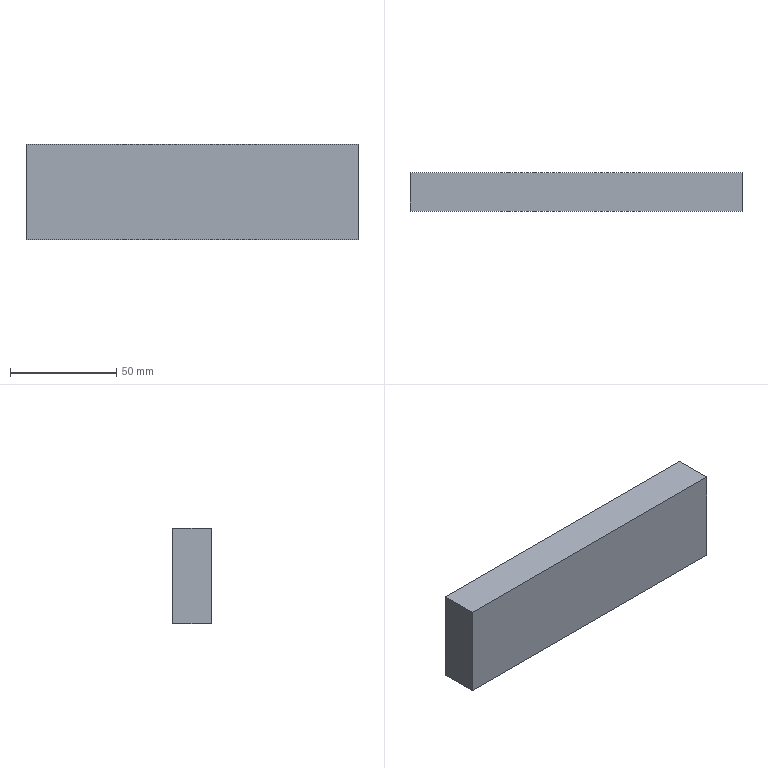Part | NX | 3 solids | 40 faces | box 156 x 18 x 45 mm | volume 213429 mm3 | plane 33 | cylinder 6 | spline 1 | commonest cylinder face diameters 6.5 x5 6 x1
STEP:
#1=CARTESIAN_POINT('',(180.,114.99,40.));
#2=VERTEX_POINT('',#1);
#3=CARTESIAN_POINT('',(30.,114.99,40.));
#4=VERTEX_POINT('',#3);
#5=CARTESIAN_POINT('',(105.,114.99,40.));
#6=DIRECTION('',(-1.,0.,0.));
#7=VECTOR('',#6,1000.);
#8=LINE('',#5,#7);
#9=EDGE_CURVE('',#2,#4,#8,.T.);
#10=ORIENTED_EDGE('',*,*,#9,.F.);
#11=CARTESIAN_POINT('',(180.,126.99,40.));
#12=VERTEX_POINT('',#11);
#13=CARTESIAN_POINT('',(180.,120.99,40.));
#14=DIRECTION('',(0.,-1.,0.));
#15=VECTOR('',#14,1000.);
#16=LINE('',#13,#15);
#17=EDGE_CURVE('',#12,#2,#16,.T.);
#18=ORIENTED_EDGE('',*,*,#17,.F.);
#19=CARTESIAN_POINT('',(30.,126.99,40.));
#20=VERTEX_POINT('',#19);
#21=CARTESIAN_POINT('',(105.,126.99,40.));
#22=DIRECTION('',(1.,0.,0.));
#23=VECTOR('',#22,1000.);
#24=LINE('',#21,#23);
#25=EDGE_CURVE('',#20,#12,#24,.T.);
#26=ORIENTED_EDGE('',*,*,#25,.F.);
#27=CARTESIAN_POINT('',(30.,120.99,40.));
#28=DIRECTION('',(0.,1.,0.));
#29=VECTOR('',#28,1000.);
#30=LINE('',#27,#29);
#31=EDGE_CURVE('',#4,#20,#30,.T.);
#32=ORIENTED_EDGE('',*,*,#31,.F.);
#33=EDGE_LOOP('',(#10,#18,#26,#32));
#34=FACE_BOUND('',#33,.T.);
#35=CARTESIAN_POINT('',(105.,120.99,40.));
#36=DIRECTION('',(0.,0.,1.));
#37=DIRECTION('',(1.,0.,0.));
#38=AXIS2_PLACEMENT_3D('',#35,#36,#37);
#39=PLANE('',#38);
#40=ADVANCED_FACE('',(#34),#39,.T.);
#41=CARTESIAN_POINT('',(180.,114.99,0.));
#42=VERTEX_POINT('',#41);
#43=CARTESIAN_POINT('',(180.,114.99,0.));
#44=DIRECTION('',(0.,0.,1.));
#45=VECTOR('',#44,1000.);
#46=LINE('',#43,#45);
#47=EDGE_CURVE('',#42,#2,#46,.T.);
#48=ORIENTED_EDGE('',*,*,#47,.T.);
#49=ORIENTED_EDGE('',*,*,#9,.T.);
#50=CARTESIAN_POINT('',(30.,114.99,0.));
#51=VERTEX_POINT('',#50);
#52=CARTESIAN_POINT('',(30.,114.99,0.));
#53=DIRECTION('',(0.,0.,1.));
#54=VECTOR('',#53,1000.);
#55=LINE('',#52,#54);
#56=EDGE_CURVE('',#51,#4,#55,.T.);
#57=ORIENTED_EDGE('',*,*,#56,.F.);
#58=CARTESIAN_POINT('',(105.,114.99,0.));
#59=DIRECTION('',(1.,0.,0.));
#60=VECTOR('',#59,1000.);
#61=LINE('',#58,#60);
#62=EDGE_CURVE('',#51,#42,#61,.T.);
#63=ORIENTED_EDGE('',*,*,#62,.T.);
#64=EDGE_LOOP('',(#48,#49,#57,#63));
#65=FACE_BOUND('',#64,.T.);
#66=CARTESIAN_POINT('',(105.,114.99,0.));
#67=DIRECTION('',(0.,-1.,0.));
#68=DIRECTION('',(0.,0.,-1.));
#69=AXIS2_PLACEMENT_3D('',#66,#67,#68);
#70=PLANE('',#69);
#71=ADVANCED_FACE('',(#65),#70,.T.);
#72=ORIENTED_EDGE('',*,*,#56,.T.);
#73=ORIENTED_EDGE('',*,*,#31,.T.);
#74=CARTESIAN_POINT('',(30.,126.99,0.));
#75=VERTEX_POINT('',#74);
#76=CARTESIAN_POINT('',(30.,126.99,0.));
#77=DIRECTION('',(0.,0.,1.));
#78=VECTOR('',#77,1000.);
#79=LINE('',#76,#78);
#80=EDGE_CURVE('',#75,#20,#79,.T.);
#81=ORIENTED_EDGE('',*,*,#80,.F.);
#82=CARTESIAN_POINT('',(30.,120.99,0.));
#83=DIRECTION('',(0.,-1.,0.));
#84=VECTOR('',#83,1000.);
#85=LINE('',#82,#84);
#86=EDGE_CURVE('',#75,#51,#85,.T.);
#87=ORIENTED_EDGE('',*,*,#86,.T.);
#88=EDGE_LOOP('',(#72,#73,#81,#87));
#89=FACE_BOUND('',#88,.T.);
#90=CARTESIAN_POINT('',(30.,120.99,0.));
#91=DIRECTION('',(-1.,0.,0.));
#92=DIRECTION('',(0.,0.,1.));
#93=AXIS2_PLACEMENT_3D('',#90,#91,#92);
#94=PLANE('',#93);
#95=ADVANCED_FACE('',(#89),#94,.T.);
#96=ORIENTED_EDGE('',*,*,#80,.T.);
#97=ORIENTED_EDGE('',*,*,#25,.T.);
#98=CARTESIAN_POINT('',(180.,126.99,0.));
#99=VERTEX_POINT('',#98);
#100=CARTESIAN_POINT('',(180.,126.99,0.));
#101=DIRECTION('',(0.,0.,1.));
#102=VECTOR('',#101,1000.);
#103=LINE('',#100,#102);
#104=EDGE_CURVE('',#99,#12,#103,.T.);
#105=ORIENTED_EDGE('',*,*,#104,.F.);
#106=CARTESIAN_POINT('',(105.,126.99,0.));
#107=DIRECTION('',(-1.,0.,0.));
#108=VECTOR('',#107,1000.);
#109=LINE('',#106,#108);
#110=EDGE_CURVE('',#99,#75,#109,.T.);
#111=ORIENTED_EDGE('',*,*,#110,.T.);
#112=EDGE_LOOP('',(#96,#97,#105,#111));
#113=FACE_BOUND('',#112,.T.);
#114=CARTESIAN_POINT('',(105.,126.99,0.));
#115=DIRECTION('',(0.,1.,0.));
#116=DIRECTION('',(0.,0.,1.));
#117=AXIS2_PLACEMENT_3D('',#114,#115,#116);
#118=PLANE('',#117);
#119=ADVANCED_FACE('',(#113),#118,.T.);
#120=CARTESIAN_POINT('',(180.,120.99,0.));
#121=DIRECTION('',(0.,1.,0.));
#122=VECTOR('',#121,1000.);
#123=LINE('',#120,#122);
#124=EDGE_CURVE('',#42,#99,#123,.T.);
#125=ORIENTED_EDGE('',*,*,#124,.F.);
#126=ORIENTED_EDGE('',*,*,#62,.F.);
#127=ORIENTED_EDGE('',*,*,#86,.F.);
#128=ORIENTED_EDGE('',*,*,#110,.F.);
#129=EDGE_LOOP('',(#125,#126,#127,#128));
#130=FACE_BOUND('',#129,.T.);
#131=CARTESIAN_POINT('',(105.,120.99,0.));
#132=DIRECTION('',(0.,0.,-1.));
#133=DIRECTION('',(-1.,0.,0.));
#134=AXIS2_PLACEMENT_3D('',#131,#132,#133);
#135=PLANE('',#134);
#136=ADVANCED_FACE('',(#130),#135,.T.);
#137=ORIENTED_EDGE('',*,*,#124,.T.);
#138=ORIENTED_EDGE('',*,*,#104,.T.);
#139=ORIENTED_EDGE('',*,*,#17,.T.);
#140=ORIENTED_EDGE('',*,*,#47,.F.);
#141=EDGE_LOOP('',(#137,#138,#139,#140));
#142=FACE_BOUND('',#141,.T.);
#143=CARTESIAN_POINT('',(180.,120.99,0.));
#144=DIRECTION('',(1.,0.,0.));
#145=DIRECTION('',(0.,0.,-1.));
#146=AXIS2_PLACEMENT_3D('',#143,#144,#145);
#147=PLANE('',#146);
#148=ADVANCED_FACE('',(#142),#147,.T.);
#149=CLOSED_SHELL('',(#40,#71,#95,#119,#136,#148));
#150=MANIFOLD_SOLID_BREP('',#149);
#151=CARTESIAN_POINT('',(175.75,115.12,7.));
#152=VERTEX_POINT('',#151);
#153=CARTESIAN_POINT('',(169.25,115.12,7.));
#154=VERTEX_POINT('',#153);
#155=CARTESIAN_POINT('',(172.5,115.12,7.));
#156=DIRECTION('',(0.,-1.,0.));
#157=DIRECTION('',(0.,0.,-1.));
#158=AXIS2_PLACEMENT_3D('',#155,#156,#157);
#159=CIRCLE('',#158,3.25);
#160=EDGE_CURVE('',#152,#154,#159,.F.);
#161=ORIENTED_EDGE('',*,*,#160,.T.);
#162=CARTESIAN_POINT('',(169.25,115.12,33.));
#163=VERTEX_POINT('',#162);
#164=CARTESIAN_POINT('',(169.25,115.12,13.));
#165=DIRECTION('',(0.,0.,1.));
#166=VECTOR('',#165,1000.);
#167=LINE('',#164,#166);
#168=EDGE_CURVE('',#154,#163,#167,.T.);
#169=ORIENTED_EDGE('',*,*,#168,.T.);
#170=CARTESIAN_POINT('',(175.75,115.12,33.));
#171=VERTEX_POINT('',#170);
#172=CARTESIAN_POINT('',(172.5,115.12,33.));
#173=DIRECTION('',(0.,-1.,0.));
#174=DIRECTION('',(0.,0.,-1.));
#175=AXIS2_PLACEMENT_3D('',#172,#173,#174);
#176=CIRCLE('',#175,3.25);
#177=EDGE_CURVE('',#163,#171,#176,.F.);
#178=ORIENTED_EDGE('',*,*,#177,.T.);
#179=CARTESIAN_POINT('',(175.75,115.12,13.));
#180=DIRECTION('',(0.,0.,-1.));
#181=VECTOR('',#180,1000.);
#182=LINE('',#179,#181);
#183=EDGE_CURVE('',#171,#152,#182,.T.);
#184=ORIENTED_EDGE('',*,*,#183,.T.);
#185=EDGE_LOOP('',(#161,#169,#178,#184));
#186=FACE_BOUND('',#185,.T.);
#187=CARTESIAN_POINT('',(165.,115.12,40.));
#188=VERTEX_POINT('',#187);
#189=CARTESIAN_POINT('',(179.,115.12,40.));
#190=VERTEX_POINT('',#189);
#191=CARTESIAN_POINT('',(158.,115.12,40.));
#192=DIRECTION('',(1.,0.,0.));
#193=VECTOR('',#192,1000.);
#194=LINE('',#191,#193);
#195=EDGE_CURVE('',#188,#190,#194,.T.);
#196=ORIENTED_EDGE('',*,*,#195,.F.);
#197=CARTESIAN_POINT('',(165.,115.12,0.));
#198=VERTEX_POINT('',#197);
#199=CARTESIAN_POINT('',(165.,115.12,13.));
#200=DIRECTION('',(0.,0.,-1.));
#201=VECTOR('',#200,1000.);
#202=LINE('',#199,#201);
#203=EDGE_CURVE('',#188,#198,#202,.T.);
#204=ORIENTED_EDGE('',*,*,#203,.T.);
#205=CARTESIAN_POINT('',(179.,115.12,0.));
#206=VERTEX_POINT('',#205);
#207=CARTESIAN_POINT('',(179.,115.12,0.));
#208=DIRECTION('',(-1.,0.,0.));
#209=VECTOR('',#208,1000.);
#210=LINE('',#207,#209);
#211=EDGE_CURVE('',#206,#198,#210,.T.);
#212=ORIENTED_EDGE('',*,*,#211,.F.);
#213=CARTESIAN_POINT('',(180.,115.12,1.));
#214=VERTEX_POINT('',#213);
#215=CARTESIAN_POINT('',(180.,115.12,1.));
#216=DIRECTION('',(-0.7071,0.,-0.7071));
#217=VECTOR('',#216,1000.);
#218=LINE('',#215,#217);
#219=EDGE_CURVE('',#214,#206,#218,.T.);
#220=ORIENTED_EDGE('',*,*,#219,.F.);
#221=CARTESIAN_POINT('',(180.,115.12,39.));
#222=VERTEX_POINT('',#221);
#223=CARTESIAN_POINT('',(180.,115.12,39.));
#224=DIRECTION('',(0.,0.,-1.));
#225=VECTOR('',#224,1000.);
#226=LINE('',#223,#225);
#227=EDGE_CURVE('',#222,#214,#226,.T.);
#228=ORIENTED_EDGE('',*,*,#227,.F.);
#229=CARTESIAN_POINT('',(179.,115.12,40.));
#230=DIRECTION('',(0.7071,0.,-0.7071));
#231=VECTOR('',#230,1000.);
#232=LINE('',#229,#231);
#233=EDGE_CURVE('',#190,#222,#232,.T.);
#234=ORIENTED_EDGE('',*,*,#233,.F.);
#235=EDGE_LOOP('',(#196,#204,#212,#220,#228,#234));
#236=FACE_BOUND('',#235,.T.);
#237=CARTESIAN_POINT('',(154.,115.12,13.));
#238=DIRECTION('',(0.,-1.,0.));
#239=DIRECTION('',(-1.,0.,0.));
#240=AXIS2_PLACEMENT_3D('',#237,#238,#239);
#241=PLANE('',#240);
#242=ADVANCED_FACE('',(#186,#236),#241,.T.);
#243=CARTESIAN_POINT('',(36.,124.24,0.));
#244=VERTEX_POINT('',#243);
#245=CARTESIAN_POINT('',(36.,117.74,0.));
#246=VERTEX_POINT('',#245);
#247=CARTESIAN_POINT('',(36.,120.99,0.));
#248=DIRECTION('',(0.,0.,1.));
#249=DIRECTION('',(1.,0.,0.));
#250=AXIS2_PLACEMENT_3D('',#247,#248,#249);
#251=CIRCLE('',#250,3.25);
#252=EDGE_CURVE('',#244,#246,#251,.T.);
#253=ORIENTED_EDGE('',*,*,#252,.T.);
#254=CARTESIAN_POINT('',(151.,117.74,0.));
#255=VERTEX_POINT('',#254);
#256=CARTESIAN_POINT('',(36.,117.74,0.));
#257=DIRECTION('',(1.,0.,0.));
#258=VECTOR('',#257,1000.);
#259=LINE('',#256,#258);
#260=EDGE_CURVE('',#246,#255,#259,.T.);
#261=ORIENTED_EDGE('',*,*,#260,.T.);
#262=CARTESIAN_POINT('',(154.,119.74,0.));
#263=VERTEX_POINT('',#262);
#264=CARTESIAN_POINT('',(151.,120.99,0.));
#265=DIRECTION('',(0.,0.,1.));
#266=DIRECTION('',(1.,0.,0.));
#267=AXIS2_PLACEMENT_3D('',#264,#265,#266);
#268=CIRCLE('',#267,3.25);
#269=EDGE_CURVE('',#255,#263,#268,.T.);
#270=ORIENTED_EDGE('',*,*,#269,.T.);
#271=CARTESIAN_POINT('',(154.,122.24,0.));
#272=VERTEX_POINT('',#271);
#273=CARTESIAN_POINT('',(154.,119.74,0.));
#274=CARTESIAN_POINT('',(154.165,120.14,0.));
#275=CARTESIAN_POINT('',(154.25,120.574,0.));
#276=CARTESIAN_POINT('',(154.25,121.406,0.));
#277=CARTESIAN_POINT('',(154.165,121.84,0.));
#278=CARTESIAN_POINT('',(154.,122.24,0.));
#279=B_SPLINE_CURVE_WITH_KNOTS('',3,(#273,#274,#275,#276,#277,#278),.UNSPECIFIED.,.F.,.F.,(4,2,4),(0.,0.5,1.),.UNSPECIFIED.);
#280=EDGE_CURVE('',#263,#272,#279,.T.);
#281=ORIENTED_EDGE('',*,*,#280,.T.);
#282=CARTESIAN_POINT('',(151.,124.24,0.));
#283=VERTEX_POINT('',#282);
#284=CARTESIAN_POINT('',(151.,120.99,0.));
#285=DIRECTION('',(0.,0.,1.));
#286=DIRECTION('',(1.,0.,0.));
#287=AXIS2_PLACEMENT_3D('',#284,#285,#286);
#288=CIRCLE('',#287,3.25);
#289=EDGE_CURVE('',#272,#283,#288,.T.);
#290=ORIENTED_EDGE('',*,*,#289,.T.);
#291=CARTESIAN_POINT('',(151.,124.24,0.));
#292=DIRECTION('',(-1.,0.,0.));
#293=VECTOR('',#292,1000.);
#294=LINE('',#291,#293);
#295=EDGE_CURVE('',#283,#244,#294,.T.);
#296=ORIENTED_EDGE('',*,*,#295,.T.);
#297=EDGE_LOOP('',(#253,#261,#270,#281,#290,#296));
#298=FACE_BOUND('',#297,.T.);
#299=ORIENTED_EDGE('',*,*,#211,.T.);
#300=CARTESIAN_POINT('',(165.,119.17,0.));
#301=VERTEX_POINT('',#300);
#302=CARTESIAN_POINT('',(165.,114.99,0.));
#303=DIRECTION('',(0.,1.,0.));
#304=VECTOR('',#303,1000.);
#305=LINE('',#302,#304);
#306=EDGE_CURVE('',#198,#301,#305,.T.);
#307=ORIENTED_EDGE('',*,*,#306,.T.);
#308=CARTESIAN_POINT('',(159.5,119.17,0.));
#309=VERTEX_POINT('',#308);
#310=CARTESIAN_POINT('',(179.,119.17,0.));
#311=DIRECTION('',(-1.,0.,0.));
#312=VECTOR('',#311,1000.);
#313=LINE('',#310,#312);
#314=EDGE_CURVE('',#301,#309,#313,.T.);
#315=ORIENTED_EDGE('',*,*,#314,.T.);
#316=CARTESIAN_POINT('',(159.5,114.99,0.));
#317=VERTEX_POINT('',#316);
#318=CARTESIAN_POINT('',(159.5,118.99,0.));
#319=DIRECTION('',(0.,-1.,0.));
#320=VECTOR('',#319,1000.);
#321=LINE('',#318,#320);
#322=EDGE_CURVE('',#309,#317,#321,.T.);
#323=ORIENTED_EDGE('',*,*,#322,.T.);
#324=CARTESIAN_POINT('',(31.,114.99,0.));
#325=VERTEX_POINT('',#324);
#326=CARTESIAN_POINT('',(179.,114.99,0.));
#327=DIRECTION('',(-1.,0.,0.));
#328=VECTOR('',#327,1000.);
#329=LINE('',#326,#328);
#330=EDGE_CURVE('',#317,#325,#329,.T.);
#331=ORIENTED_EDGE('',*,*,#330,.T.);
#332=CARTESIAN_POINT('',(31.,126.99,0.));
#333=VERTEX_POINT('',#332);
#334=CARTESIAN_POINT('',(31.,114.99,0.));
#335=DIRECTION('',(0.,1.,0.));
#336=VECTOR('',#335,1000.);
#337=LINE('',#334,#336);
#338=EDGE_CURVE('',#325,#333,#337,.T.);
#339=ORIENTED_EDGE('',*,*,#338,.T.);
#340=CARTESIAN_POINT('',(179.,126.99,0.));
#341=VERTEX_POINT('',#340);
#342=CARTESIAN_POINT('',(179.,126.99,0.));
#343=DIRECTION('',(-1.,0.,0.));
#344=VECTOR('',#343,1000.);
#345=LINE('',#342,#344);
#346=EDGE_CURVE('',#341,#333,#345,.T.);
#347=ORIENTED_EDGE('',*,*,#346,.F.);
#348=CARTESIAN_POINT('',(179.,114.99,0.));
#349=DIRECTION('',(0.,1.,0.));
#350=VECTOR('',#349,1000.);
#351=LINE('',#348,#350);
#352=EDGE_CURVE('',#206,#341,#351,.T.);
#353=ORIENTED_EDGE('',*,*,#352,.F.);
#354=EDGE_LOOP('',(#299,#307,#315,#323,#331,#339,#347,#353));
#355=FACE_BOUND('',#354,.T.);
#356=CARTESIAN_POINT('',(179.,114.99,0.));
#357=DIRECTION('',(0.,0.,-1.));
#358=DIRECTION('',(0.,1.,0.));
#359=AXIS2_PLACEMENT_3D('',#356,#357,#358);
#360=PLANE('',#359);
#361=ADVANCED_FACE('',(#298,#355),#360,.T.);
#362=CARTESIAN_POINT('',(154.,122.24,10.));
#363=VERTEX_POINT('',#362);
#364=CARTESIAN_POINT('',(154.,126.99,10.));
#365=VERTEX_POINT('',#364);
#366=CARTESIAN_POINT('',(154.,114.99,10.));
#367=DIRECTION('',(0.,1.,0.));
#368=VECTOR('',#367,1000.);
#369=LINE('',#366,#368);
#370=EDGE_CURVE('',#363,#365,#369,.T.);
#371=ORIENTED_EDGE('',*,*,#370,.F.);
#372=CARTESIAN_POINT('',(154.,119.74,10.));
#373=VERTEX_POINT('',#372);
#374=CARTESIAN_POINT('',(154.,122.24,10.));
#375=CARTESIAN_POINT('',(154.329,121.445,10.));
#376=CARTESIAN_POINT('',(154.329,120.536,10.));
#377=CARTESIAN_POINT('',(154.,119.74,10.));
#378=B_SPLINE_CURVE_WITH_KNOTS('',3,(#374,#375,#376,#377),.UNSPECIFIED.,.F.,.F.,(4,4),(0.,0.002569),.UNSPECIFIED.);
#379=EDGE_CURVE('',#363,#373,#378,.T.);
#380=ORIENTED_EDGE('',*,*,#379,.T.);
#381=CARTESIAN_POINT('',(154.,114.99,10.));
#382=VERTEX_POINT('',#381);
#383=CARTESIAN_POINT('',(154.,114.99,10.));
#384=DIRECTION('',(0.,1.,0.));
#385=VECTOR('',#384,1000.);
#386=LINE('',#383,#385);
#387=EDGE_CURVE('',#382,#373,#386,.T.);
#388=ORIENTED_EDGE('',*,*,#387,.F.);
#389=CARTESIAN_POINT('',(157.,114.99,13.));
#390=VERTEX_POINT('',#389);
#391=CARTESIAN_POINT('',(154.,114.99,13.));
#392=DIRECTION('',(0.,-1.,0.));
#393=DIRECTION('',(1.,0.,0.));
#394=AXIS2_PLACEMENT_3D('',#391,#392,#393);
#395=CIRCLE('',#394,3.);
#396=EDGE_CURVE('',#382,#390,#395,.T.);
#397=ORIENTED_EDGE('',*,*,#396,.T.);
#398=CARTESIAN_POINT('',(157.,126.99,13.));
#399=VERTEX_POINT('',#398);
#400=CARTESIAN_POINT('',(157.,114.99,13.));
#401=DIRECTION('',(0.,1.,0.));
#402=VECTOR('',#401,1000.);
#403=LINE('',#400,#402);
#404=EDGE_CURVE('',#390,#399,#403,.T.);
#405=ORIENTED_EDGE('',*,*,#404,.T.);
#406=CARTESIAN_POINT('',(154.,126.99,13.));
#407=DIRECTION('',(0.,-1.,0.));
#408=DIRECTION('',(1.,0.,0.));
#409=AXIS2_PLACEMENT_3D('',#406,#407,#408);
#410=CIRCLE('',#409,3.);
#411=EDGE_CURVE('',#365,#399,#410,.T.);
#412=ORIENTED_EDGE('',*,*,#411,.F.);
#413=EDGE_LOOP('',(#371,#380,#388,#397,#405,#412));
#414=FACE_BOUND('',#413,.T.);
#415=CARTESIAN_POINT('',(154.,114.99,13.));
#416=DIRECTION('',(0.,1.,0.));
#417=DIRECTION('',(1.,0.,0.));
#418=AXIS2_PLACEMENT_3D('',#415,#416,#417);
#419=CYLINDRICAL_SURFACE('',#418,3.);
#420=ADVANCED_FACE('',(#414),#419,.F.);
#421=ORIENTED_EDGE('',*,*,#387,.T.);
#422=CARTESIAN_POINT('',(151.,117.74,10.));
#423=VERTEX_POINT('',#422);
#424=CARTESIAN_POINT('',(151.,120.99,10.));
#425=DIRECTION('',(0.,0.,1.));
#426=DIRECTION('',(1.,0.,0.));
#427=AXIS2_PLACEMENT_3D('',#424,#425,#426);
#428=CIRCLE('',#427,3.25);
#429=EDGE_CURVE('',#373,#423,#428,.F.);
#430=ORIENTED_EDGE('',*,*,#429,.T.);
#431=CARTESIAN_POINT('',(36.,117.74,10.));
#432=VERTEX_POINT('',#431);
#433=CARTESIAN_POINT('',(31.,117.74,10.));
#434=DIRECTION('',(-1.,0.,0.));
#435=VECTOR('',#434,1000.);
#436=LINE('',#433,#435);
#437=EDGE_CURVE('',#423,#432,#436,.T.);
#438=ORIENTED_EDGE('',*,*,#437,.T.);
#439=CARTESIAN_POINT('',(36.,124.24,10.));
#440=VERTEX_POINT('',#439);
#441=CARTESIAN_POINT('',(36.,120.99,10.));
#442=DIRECTION('',(0.,0.,1.));
#443=DIRECTION('',(1.,0.,0.));
#444=AXIS2_PLACEMENT_3D('',#441,#442,#443);
#445=CIRCLE('',#444,3.25);
#446=EDGE_CURVE('',#432,#440,#445,.F.);
#447=ORIENTED_EDGE('',*,*,#446,.T.);
#448=CARTESIAN_POINT('',(151.,124.24,10.));
#449=VERTEX_POINT('',#448);
#450=CARTESIAN_POINT('',(31.,124.24,10.));
#451=DIRECTION('',(1.,0.,0.));
#452=VECTOR('',#451,1000.);
#453=LINE('',#450,#452);
#454=EDGE_CURVE('',#440,#449,#453,.T.);
#455=ORIENTED_EDGE('',*,*,#454,.T.);
#456=CARTESIAN_POINT('',(151.,120.99,10.));
#457=DIRECTION('',(0.,0.,1.));
#458=DIRECTION('',(1.,0.,0.));
#459=AXIS2_PLACEMENT_3D('',#456,#457,#458);
#460=CIRCLE('',#459,3.25);
#461=EDGE_CURVE('',#449,#363,#460,.F.);
#462=ORIENTED_EDGE('',*,*,#461,.T.);
#463=ORIENTED_EDGE('',*,*,#370,.T.);
#464=CARTESIAN_POINT('',(31.,126.99,10.));
#465=VERTEX_POINT('',#464);
#466=CARTESIAN_POINT('',(31.,126.99,10.));
#467=DIRECTION('',(1.,0.,0.));
#468=VECTOR('',#467,1000.);
#469=LINE('',#466,#468);
#470=EDGE_CURVE('',#465,#365,#469,.T.);
#471=ORIENTED_EDGE('',*,*,#470,.F.);
#472=CARTESIAN_POINT('',(31.,114.99,10.));
#473=VERTEX_POINT('',#472);
#474=CARTESIAN_POINT('',(31.,114.99,10.));
#475=DIRECTION('',(0.,1.,0.));
#476=VECTOR('',#475,1000.);
#477=LINE('',#474,#476);
#478=EDGE_CURVE('',#473,#465,#477,.T.);
#479=ORIENTED_EDGE('',*,*,#478,.F.);
#480=CARTESIAN_POINT('',(31.,114.99,10.));
#481=DIRECTION('',(1.,0.,0.));
#482=VECTOR('',#481,1000.);
#483=LINE('',#480,#482);
#484=EDGE_CURVE('',#473,#382,#483,.T.);
#485=ORIENTED_EDGE('',*,*,#484,.T.);
#486=EDGE_LOOP('',(#421,#430,#438,#447,#455,#462,#463,#471,#479,#485));
#487=FACE_BOUND('',#486,.T.);
#488=CARTESIAN_POINT('',(31.,114.99,10.));
#489=DIRECTION('',(0.,0.,1.));
#490=DIRECTION('',(1.,0.,0.));
#491=AXIS2_PLACEMENT_3D('',#488,#489,#490);
#492=PLANE('',#491);
#493=ADVANCED_FACE('',(#487),#492,.T.);
#494=CARTESIAN_POINT('',(157.,126.99,39.));
#495=VERTEX_POINT('',#494);
#496=CARTESIAN_POINT('',(157.,126.99,13.));
#497=DIRECTION('',(0.,0.,1.));
#498=VECTOR('',#497,1000.);
#499=LINE('',#496,#498);
#500=EDGE_CURVE('',#399,#495,#499,.T.);
#501=ORIENTED_EDGE('',*,*,#500,.F.);
#502=ORIENTED_EDGE('',*,*,#404,.F.);
#503=CARTESIAN_POINT('',(157.,114.99,39.));
#504=VERTEX_POINT('',#503);
#505=CARTESIAN_POINT('',(157.,114.99,13.));
#506=DIRECTION('',(0.,0.,1.));
#507=VECTOR('',#506,1000.);
#508=LINE('',#505,#507);
#509=EDGE_CURVE('',#390,#504,#508,.T.);
#510=ORIENTED_EDGE('',*,*,#509,.T.);
#511=CARTESIAN_POINT('',(157.,114.99,39.));
#512=DIRECTION('',(0.,1.,0.));
#513=VECTOR('',#512,1000.);
#514=LINE('',#511,#513);
#515=EDGE_CURVE('',#504,#495,#514,.T.);
#516=ORIENTED_EDGE('',*,*,#515,.T.);
#517=EDGE_LOOP('',(#501,#502,#510,#516));
#518=FACE_BOUND('',#517,.T.);
#519=CARTESIAN_POINT('',(157.,114.99,13.));
#520=DIRECTION('',(-1.,0.,0.));
#521=DIRECTION('',(0.,1.,0.));
#522=AXIS2_PLACEMENT_3D('',#519,#520,#521);
#523=PLANE('',#522);
#524=ADVANCED_FACE('',(#518),#523,.T.);
#525=CARTESIAN_POINT('',(158.,126.99,40.));
#526=VERTEX_POINT('',#525);
#527=CARTESIAN_POINT('',(157.,126.99,39.));
#528=DIRECTION('',(0.7071,0.,0.7071));
#529=VECTOR('',#528,1000.);
#530=LINE('',#527,#529);
#531=EDGE_CURVE('',#495,#526,#530,.T.);
#532=ORIENTED_EDGE('',*,*,#531,.F.);
#533=ORIENTED_EDGE('',*,*,#515,.F.);
#534=CARTESIAN_POINT('',(158.,114.99,40.));
#535=VERTEX_POINT('',#534);
#536=CARTESIAN_POINT('',(157.,114.99,39.));
#537=DIRECTION('',(0.7071,0.,0.7071));
#538=VECTOR('',#537,1000.);
#539=LINE('',#536,#538);
#540=EDGE_CURVE('',#504,#535,#539,.T.);
#541=ORIENTED_EDGE('',*,*,#540,.T.);
#542=CARTESIAN_POINT('',(158.,114.99,40.));
#543=DIRECTION('',(0.,1.,0.));
#544=VECTOR('',#543,1000.);
#545=LINE('',#542,#544);
#546=EDGE_CURVE('',#535,#526,#545,.T.);
#547=ORIENTED_EDGE('',*,*,#546,.T.);
#548=EDGE_LOOP('',(#532,#533,#541,#547));
#549=FACE_BOUND('',#548,.T.);
#550=CARTESIAN_POINT('',(157.,114.99,39.));
#551=DIRECTION('',(-0.7071,0.,0.7071));
#552=DIRECTION('',(0.7071,0.,0.7071));
#553=AXIS2_PLACEMENT_3D('',#550,#551,#552);
#554=PLANE('',#553);
#555=ADVANCED_FACE('',(#549),#554,.T.);
#556=CARTESIAN_POINT('',(159.5,119.17,40.));
#557=VERTEX_POINT('',#556);
#558=CARTESIAN_POINT('',(159.5,114.99,40.));
#559=VERTEX_POINT('',#558);
#560=CARTESIAN_POINT('',(159.5,118.99,40.));
#561=DIRECTION('',(0.,-1.,0.));
#562=VECTOR('',#561,1000.);
#563=LINE('',#560,#562);
#564=EDGE_CURVE('',#557,#559,#563,.T.);
#565=ORIENTED_EDGE('',*,*,#564,.F.);
#566=CARTESIAN_POINT('',(165.,119.17,40.));
#567=VERTEX_POINT('',#566);
#568=CARTESIAN_POINT('',(165.,119.17,40.));
#569=DIRECTION('',(-1.,0.,0.));
#570=VECTOR('',#569,1000.);
#571=LINE('',#568,#570);
#572=EDGE_CURVE('',#567,#557,#571,.T.);
#573=ORIENTED_EDGE('',*,*,#572,.F.);
#574=CARTESIAN_POINT('',(165.,114.99,40.));
#575=DIRECTION('',(0.,1.,0.));
#576=VECTOR('',#575,1000.);
#577=LINE('',#574,#576);
#578=EDGE_CURVE('',#188,#567,#577,.T.);
#579=ORIENTED_EDGE('',*,*,#578,.F.);
#580=ORIENTED_EDGE('',*,*,#195,.T.);
#581=CARTESIAN_POINT('',(179.,126.99,40.));
#582=VERTEX_POINT('',#581);
#583=CARTESIAN_POINT('',(179.,114.99,40.));
#584=DIRECTION('',(0.,1.,0.));
#585=VECTOR('',#584,1000.);
#586=LINE('',#583,#585);
#587=EDGE_CURVE('',#190,#582,#586,.T.);
#588=ORIENTED_EDGE('',*,*,#587,.T.);
#589=CARTESIAN_POINT('',(158.,126.99,40.));
#590=DIRECTION('',(1.,0.,0.));
#591=VECTOR('',#590,1000.);
#592=LINE('',#589,#591);
#593=EDGE_CURVE('',#526,#582,#592,.T.);
#594=ORIENTED_EDGE('',*,*,#593,.F.);
#595=ORIENTED_EDGE('',*,*,#546,.F.);
#596=CARTESIAN_POINT('',(158.,114.99,40.));
#597=DIRECTION('',(1.,0.,0.));
#598=VECTOR('',#597,1000.);
#599=LINE('',#596,#598);
#600=EDGE_CURVE('',#535,#559,#599,.T.);
#601=ORIENTED_EDGE('',*,*,#600,.T.);
#602=EDGE_LOOP('',(#565,#573,#579,#580,#588,#594,#595,#601));
#603=FACE_BOUND('',#602,.T.);
#604=CARTESIAN_POINT('',(158.,114.99,40.));
#605=DIRECTION('',(0.,0.,1.));
#606=DIRECTION('',(0.,-1.,0.));
#607=AXIS2_PLACEMENT_3D('',#604,#605,#606);
#608=PLANE('',#607);
#609=ADVANCED_FACE('',(#603),#608,.T.);
#610=CARTESIAN_POINT('',(180.,126.99,39.));
#611=VERTEX_POINT('',#610);
#612=CARTESIAN_POINT('',(179.,126.99,40.));
#613=DIRECTION('',(0.7071,0.,-0.7071));
#614=VECTOR('',#613,1000.);
#615=LINE('',#612,#614);
#616=EDGE_CURVE('',#582,#611,#615,.T.);
#617=ORIENTED_EDGE('',*,*,#616,.F.);
#618=ORIENTED_EDGE('',*,*,#587,.F.);
#619=ORIENTED_EDGE('',*,*,#233,.T.);
#620=CARTESIAN_POINT('',(180.,114.99,39.));
#621=DIRECTION('',(0.,1.,0.));
#622=VECTOR('',#621,1000.);
#623=LINE('',#620,#622);
#624=EDGE_CURVE('',#222,#611,#623,.T.);
#625=ORIENTED_EDGE('',*,*,#624,.T.);
#626=EDGE_LOOP('',(#617,#618,#619,#625));
#627=FACE_BOUND('',#626,.T.);
#628=CARTESIAN_POINT('',(179.,114.99,40.));
#629=DIRECTION('',(0.7071,0.,0.7071));
#630=DIRECTION('',(0.7071,0.,-0.7071));
#631=AXIS2_PLACEMENT_3D('',#628,#629,#630);
#632=PLANE('',#631);
#633=ADVANCED_FACE('',(#627),#632,.T.);
#634=CARTESIAN_POINT('',(180.,126.99,1.));
#635=VERTEX_POINT('',#634);
#636=CARTESIAN_POINT('',(180.,126.99,39.));
#637=DIRECTION('',(0.,0.,-1.));
#638=VECTOR('',#637,1000.);
#639=LINE('',#636,#638);
#640=EDGE_CURVE('',#611,#635,#639,.T.);
#641=ORIENTED_EDGE('',*,*,#640,.F.);
#642=ORIENTED_EDGE('',*,*,#624,.F.);
#643=ORIENTED_EDGE('',*,*,#227,.T.);
#644=CARTESIAN_POINT('',(180.,114.99,1.));
#645=DIRECTION('',(0.,1.,0.));
#646=VECTOR('',#645,1000.);
#647=LINE('',#644,#646);
#648=EDGE_CURVE('',#214,#635,#647,.T.);
#649=ORIENTED_EDGE('',*,*,#648,.T.);
#650=EDGE_LOOP('',(#641,#642,#643,#649));
#651=FACE_BOUND('',#650,.T.);
#652=CARTESIAN_POINT('',(180.,114.99,39.));
#653=DIRECTION('',(1.,0.,0.));
#654=DIRECTION('',(0.,-1.,0.));
#655=AXIS2_PLACEMENT_3D('',#652,#653,#654);
#656=PLANE('',#655);
#657=ADVANCED_FACE('',(#651),#656,.T.);
#658=CARTESIAN_POINT('',(180.,126.99,1.));
#659=DIRECTION('',(-0.7071,0.,-0.7071));
#660=VECTOR('',#659,1000.);
#661=LINE('',#658,#660);
#662=EDGE_CURVE('',#635,#341,#661,.T.);
#663=ORIENTED_EDGE('',*,*,#662,.F.);
#664=ORIENTED_EDGE('',*,*,#648,.F.);
#665=ORIENTED_EDGE('',*,*,#219,.T.);
#666=ORIENTED_EDGE('',*,*,#352,.T.);
#667=EDGE_LOOP('',(#663,#664,#665,#666));
#668=FACE_BOUND('',#667,.T.);
#669=CARTESIAN_POINT('',(180.,114.99,1.));
#670=DIRECTION('',(0.7071,0.,-0.7071));
#671=DIRECTION('',(-0.7071,0.,-0.7071));
#672=AXIS2_PLACEMENT_3D('',#669,#670,#671);
#673=PLANE('',#672);
#674=ADVANCED_FACE('',(#668),#673,.T.);
#675=CARTESIAN_POINT('',(30.,126.99,1.));
#676=VERTEX_POINT('',#675);
#677=CARTESIAN_POINT('',(31.,126.99,0.));
#678=DIRECTION('',(-0.7071,0.,0.7071));
#679=VECTOR('',#678,1000.);
#680=LINE('',#677,#679);
#681=EDGE_CURVE('',#333,#676,#680,.T.);
#682=ORIENTED_EDGE('',*,*,#681,.F.);
#683=ORIENTED_EDGE('',*,*,#338,.F.);
#684=CARTESIAN_POINT('',(30.,114.99,1.));
#685=VERTEX_POINT('',#684);
#686=CARTESIAN_POINT('',(31.,114.99,0.));
#687=DIRECTION('',(-0.7071,0.,0.7071));
#688=VECTOR('',#687,1000.);
#689=LINE('',#686,#688);
#690=EDGE_CURVE('',#325,#685,#689,.T.);
#691=ORIENTED_EDGE('',*,*,#690,.T.);
#692=CARTESIAN_POINT('',(30.,114.99,1.));
#693=DIRECTION('',(0.,1.,0.));
#694=VECTOR('',#693,1000.);
#695=LINE('',#692,#694);
#696=EDGE_CURVE('',#685,#676,#695,.T.);
#697=ORIENTED_EDGE('',*,*,#696,.T.);
#698=EDGE_LOOP('',(#682,#683,#691,#697));
#699=FACE_BOUND('',#698,.T.);
#700=CARTESIAN_POINT('',(31.,114.99,0.));
#701=DIRECTION('',(-0.7071,0.,-0.7071));
#702=DIRECTION('',(-0.7071,0.,0.7071));
#703=AXIS2_PLACEMENT_3D('',#700,#701,#702);
#704=PLANE('',#703);
#705=ADVANCED_FACE('',(#699),#704,.T.);
#706=CARTESIAN_POINT('',(30.,126.99,9.));
#707=VERTEX_POINT('',#706);
#708=CARTESIAN_POINT('',(30.,126.99,1.));
#709=DIRECTION('',(0.,0.,1.));
#710=VECTOR('',#709,1000.);
#711=LINE('',#708,#710);
#712=EDGE_CURVE('',#676,#707,#711,.T.);
#713=ORIENTED_EDGE('',*,*,#712,.F.);
#714=ORIENTED_EDGE('',*,*,#696,.F.);
#715=CARTESIAN_POINT('',(30.,114.99,9.));
#716=VERTEX_POINT('',#715);
#717=CARTESIAN_POINT('',(30.,114.99,1.));
#718=DIRECTION('',(0.,0.,1.));
#719=VECTOR('',#718,1000.);
#720=LINE('',#717,#719);
#721=EDGE_CURVE('',#685,#716,#720,.T.);
#722=ORIENTED_EDGE('',*,*,#721,.T.);
#723=CARTESIAN_POINT('',(30.,114.99,9.));
#724=DIRECTION('',(0.,1.,0.));
#725=VECTOR('',#724,1000.);
#726=LINE('',#723,#725);
#727=EDGE_CURVE('',#716,#707,#726,.T.);
#728=ORIENTED_EDGE('',*,*,#727,.T.);
#729=EDGE_LOOP('',(#713,#714,#722,#728));
#730=FACE_BOUND('',#729,.T.);
#731=CARTESIAN_POINT('',(30.,114.99,1.));
#732=DIRECTION('',(-1.,0.,0.));
#733=DIRECTION('',(0.,1.,0.));
#734=AXIS2_PLACEMENT_3D('',#731,#732,#733);
#735=PLANE('',#734);
#736=ADVANCED_FACE('',(#730),#735,.T.);
#737=CARTESIAN_POINT('',(30.,126.99,9.));
#738=DIRECTION('',(0.7071,0.,0.7071));
#739=VECTOR('',#738,1000.);
#740=LINE('',#737,#739);
#741=EDGE_CURVE('',#707,#465,#740,.T.);
#742=ORIENTED_EDGE('',*,*,#741,.F.);
#743=ORIENTED_EDGE('',*,*,#727,.F.);
#744=CARTESIAN_POINT('',(30.,114.99,9.));
#745=DIRECTION('',(0.7071,0.,0.7071));
#746=VECTOR('',#745,1000.);
#747=LINE('',#744,#746);
#748=EDGE_CURVE('',#716,#473,#747,.T.);
#749=ORIENTED_EDGE('',*,*,#748,.T.);
#750=ORIENTED_EDGE('',*,*,#478,.T.);
#751=EDGE_LOOP('',(#742,#743,#749,#750));
#752=FACE_BOUND('',#751,.T.);
#753=CARTESIAN_POINT('',(30.,114.99,9.));
#754=DIRECTION('',(-0.7071,0.,0.7071));
#755=DIRECTION('',(0.7071,0.,0.7071));
#756=AXIS2_PLACEMENT_3D('',#753,#754,#755);
#757=PLANE('',#756);
#758=ADVANCED_FACE('',(#752),#757,.T.);
#759=CARTESIAN_POINT('',(159.5,114.99,40.));
#760=DIRECTION('',(0.,0.,-1.));
#761=VECTOR('',#760,1000.);
#762=LINE('',#759,#761);
#763=EDGE_CURVE('',#559,#317,#762,.T.);
#764=ORIENTED_EDGE('',*,*,#763,.F.);
#765=ORIENTED_EDGE('',*,*,#600,.F.);
#766=ORIENTED_EDGE('',*,*,#540,.F.);
#767=ORIENTED_EDGE('',*,*,#509,.F.);
#768=ORIENTED_EDGE('',*,*,#396,.F.);
#769=ORIENTED_EDGE('',*,*,#484,.F.);
#770=ORIENTED_EDGE('',*,*,#748,.F.);
#771=ORIENTED_EDGE('',*,*,#721,.F.);
#772=ORIENTED_EDGE('',*,*,#690,.F.);
#773=ORIENTED_EDGE('',*,*,#330,.F.);
#774=EDGE_LOOP('',(#764,#765,#766,#767,#768,#769,#770,#771,#772,#773));
#775=FACE_BOUND('',#774,.T.);
#776=CARTESIAN_POINT('',(154.,114.99,13.));
#777=DIRECTION('',(0.,-1.,0.));
#778=DIRECTION('',(-1.,0.,0.));
#779=AXIS2_PLACEMENT_3D('',#776,#777,#778);
#780=PLANE('',#779);
#781=ADVANCED_FACE('',(#775),#780,.T.);
#782=CARTESIAN_POINT('',(169.25,126.99,33.));
#783=VERTEX_POINT('',#782);
#784=CARTESIAN_POINT('',(169.25,126.99,7.));
#785=VERTEX_POINT('',#784);
#786=CARTESIAN_POINT('',(169.25,126.99,33.));
#787=DIRECTION('',(0.,0.,-1.));
#788=VECTOR('',#787,1000.);
#789=LINE('',#786,#788);
#790=EDGE_CURVE('',#783,#785,#789,.T.);
#791=ORIENTED_EDGE('',*,*,#790,.T.);
#792=CARTESIAN_POINT('',(175.75,126.99,7.));
#793=VERTEX_POINT('',#792);
#794=CARTESIAN_POINT('',(172.5,126.99,7.));
#795=DIRECTION('',(0.,-1.,0.));
#796=DIRECTION('',(1.,0.,0.));
#797=AXIS2_PLACEMENT_3D('',#794,#795,#796);
#798=CIRCLE('',#797,3.25);
#799=EDGE_CURVE('',#785,#793,#798,.T.);
#800=ORIENTED_EDGE('',*,*,#799,.T.);
#801=CARTESIAN_POINT('',(175.75,126.99,33.));
#802=VERTEX_POINT('',#801);
#803=CARTESIAN_POINT('',(175.75,126.99,7.));
#804=DIRECTION('',(0.,0.,1.));
#805=VECTOR('',#804,1000.);
#806=LINE('',#803,#805);
#807=EDGE_CURVE('',#793,#802,#806,.T.);
#808=ORIENTED_EDGE('',*,*,#807,.T.);
#809=CARTESIAN_POINT('',(172.5,126.99,33.));
#810=DIRECTION('',(0.,-1.,0.));
#811=DIRECTION('',(1.,0.,0.));
#812=AXIS2_PLACEMENT_3D('',#809,#810,#811);
#813=CIRCLE('',#812,3.25);
#814=EDGE_CURVE('',#802,#783,#813,.T.);
#815=ORIENTED_EDGE('',*,*,#814,.T.);
#816=EDGE_LOOP('',(#791,#800,#808,#815));
#817=FACE_BOUND('',#816,.T.);
#818=ORIENTED_EDGE('',*,*,#470,.T.);
#819=ORIENTED_EDGE('',*,*,#411,.T.);
#820=ORIENTED_EDGE('',*,*,#500,.T.);
#821=ORIENTED_EDGE('',*,*,#531,.T.);
#822=ORIENTED_EDGE('',*,*,#593,.T.);
#823=ORIENTED_EDGE('',*,*,#616,.T.);
#824=ORIENTED_EDGE('',*,*,#640,.T.);
#825=ORIENTED_EDGE('',*,*,#662,.T.);
#826=ORIENTED_EDGE('',*,*,#346,.T.);
#827=ORIENTED_EDGE('',*,*,#681,.T.);
#828=ORIENTED_EDGE('',*,*,#712,.T.);
#829=ORIENTED_EDGE('',*,*,#741,.T.);
#830=EDGE_LOOP('',(#818,#819,#820,#821,#822,#823,#824,#825,#826,#827,#828,#829));
#831=FACE_BOUND('',#830,.T.);
#832=CARTESIAN_POINT('',(154.,126.99,13.));
#833=DIRECTION('',(0.,-1.,0.));
#834=DIRECTION('',(-1.,0.,0.));
#835=AXIS2_PLACEMENT_3D('',#832,#833,#834);
#836=PLANE('',#835);
#837=ADVANCED_FACE('',(#817,#831),#836,.F.);
#838=CARTESIAN_POINT('',(169.25,86.99,7.));
#839=DIRECTION('',(0.,1.,0.));
#840=VECTOR('',#839,1000.);
#841=LINE('',#838,#840);
#842=EDGE_CURVE('',#785,#154,#841,.F.);
#843=ORIENTED_EDGE('',*,*,#842,.F.);
#844=ORIENTED_EDGE('',*,*,#790,.F.);
#845=CARTESIAN_POINT('',(169.25,86.99,33.));
#846=DIRECTION('',(0.,1.,0.));
#847=VECTOR('',#846,1000.);
#848=LINE('',#845,#847);
#849=EDGE_CURVE('',#783,#163,#848,.F.);
#850=ORIENTED_EDGE('',*,*,#849,.T.);
#851=ORIENTED_EDGE('',*,*,#168,.F.);
#852=EDGE_LOOP('',(#843,#844,#850,#851));
#853=FACE_BOUND('',#852,.T.);
#854=CARTESIAN_POINT('',(169.25,86.99,33.));
#855=DIRECTION('',(1.,0.,0.));
#856=DIRECTION('',(0.,0.,-1.));
#857=AXIS2_PLACEMENT_3D('',#854,#855,#856);
#858=PLANE('',#857);
#859=ADVANCED_FACE('',(#853),#858,.T.);
#860=CARTESIAN_POINT('',(175.75,86.99,7.));
#861=DIRECTION('',(0.,1.,0.));
#862=VECTOR('',#861,1000.);
#863=LINE('',#860,#862);
#864=EDGE_CURVE('',#793,#152,#863,.F.);
#865=ORIENTED_EDGE('',*,*,#864,.F.);
#866=ORIENTED_EDGE('',*,*,#799,.F.);
#867=ORIENTED_EDGE('',*,*,#842,.T.);
#868=ORIENTED_EDGE('',*,*,#160,.F.);
#869=EDGE_LOOP('',(#865,#866,#867,#868));
#870=FACE_BOUND('',#869,.T.);
#871=CARTESIAN_POINT('',(172.5,86.99,7.));
#872=DIRECTION('',(0.,1.,0.));
#873=DIRECTION('',(1.,0.,0.));
#874=AXIS2_PLACEMENT_3D('',#871,#872,#873);
#875=CYLINDRICAL_SURFACE('',#874,3.25);
#876=ADVANCED_FACE('',(#870),#875,.F.);
#877=CARTESIAN_POINT('',(175.75,86.99,33.));
#878=DIRECTION('',(0.,1.,0.));
#879=VECTOR('',#878,1000.);
#880=LINE('',#877,#879);
#881=EDGE_CURVE('',#802,#171,#880,.F.);
#882=ORIENTED_EDGE('',*,*,#881,.F.);
#883=ORIENTED_EDGE('',*,*,#807,.F.);
#884=ORIENTED_EDGE('',*,*,#864,.T.);
#885=ORIENTED_EDGE('',*,*,#183,.F.);
#886=EDGE_LOOP('',(#882,#883,#884,#885));
#887=FACE_BOUND('',#886,.T.);
#888=CARTESIAN_POINT('',(175.75,86.99,7.));
#889=DIRECTION('',(-1.,0.,0.));
#890=DIRECTION('',(0.,0.,1.));
#891=AXIS2_PLACEMENT_3D('',#888,#889,#890);
#892=PLANE('',#891);
#893=ADVANCED_FACE('',(#887),#892,.T.);
#894=ORIENTED_EDGE('',*,*,#849,.F.);
#895=ORIENTED_EDGE('',*,*,#814,.F.);
#896=ORIENTED_EDGE('',*,*,#881,.T.);
#897=ORIENTED_EDGE('',*,*,#177,.F.);
#898=EDGE_LOOP('',(#894,#895,#896,#897));
#899=FACE_BOUND('',#898,.T.);
#900=CARTESIAN_POINT('',(172.5,86.99,33.));
#901=DIRECTION('',(0.,1.,0.));
#902=DIRECTION('',(1.,0.,0.));
#903=AXIS2_PLACEMENT_3D('',#900,#901,#902);
#904=CYLINDRICAL_SURFACE('',#903,3.25);
#905=ADVANCED_FACE('',(#899),#904,.F.);
#906=CARTESIAN_POINT('',(151.,117.74,40.));
#907=DIRECTION('',(0.,0.,-1.));
#908=VECTOR('',#907,1000.);
#909=LINE('',#906,#908);
#910=EDGE_CURVE('',#423,#255,#909,.T.);
#911=ORIENTED_EDGE('',*,*,#910,.T.);
#912=ORIENTED_EDGE('',*,*,#260,.F.);
#913=CARTESIAN_POINT('',(36.,117.74,40.));
#914=DIRECTION('',(0.,0.,-1.));
#915=VECTOR('',#914,1000.);
#916=LINE('',#913,#915);
#917=EDGE_CURVE('',#432,#246,#916,.T.);
#918=ORIENTED_EDGE('',*,*,#917,.F.);
#919=ORIENTED_EDGE('',*,*,#437,.F.);
#920=EDGE_LOOP('',(#911,#912,#918,#919));
#921=FACE_BOUND('',#920,.T.);
#922=CARTESIAN_POINT('',(36.,117.74,40.));
#923=DIRECTION('',(0.,1.,0.));
#924=DIRECTION('',(-1.,0.,0.));
#925=AXIS2_PLACEMENT_3D('',#922,#923,#924);
#926=PLANE('',#925);
#927=ADVANCED_FACE('',(#921),#926,.T.);
#928=CARTESIAN_POINT('',(154.,119.74,40.));
#929=DIRECTION('',(0.,0.,-1.));
#930=VECTOR('',#929,1000.);
#931=LINE('',#928,#930);
#932=EDGE_CURVE('',#373,#263,#931,.T.);
#933=ORIENTED_EDGE('',*,*,#932,.T.);
#934=ORIENTED_EDGE('',*,*,#269,.F.);
#935=ORIENTED_EDGE('',*,*,#910,.F.);
#936=ORIENTED_EDGE('',*,*,#429,.F.);
#937=EDGE_LOOP('',(#933,#934,#935,#936));
#938=FACE_BOUND('',#937,.T.);
#939=CARTESIAN_POINT('',(151.,120.99,40.));
#940=DIRECTION('',(0.,0.,-1.));
#941=DIRECTION('',(-1.,0.,0.));
#942=AXIS2_PLACEMENT_3D('',#939,#940,#941);
#943=CYLINDRICAL_SURFACE('',#942,3.25);
#944=ADVANCED_FACE('',(#938),#943,.F.);
#945=CARTESIAN_POINT('',(154.,122.24,40.));
#946=DIRECTION('',(0.,0.,-1.));
#947=VECTOR('',#946,1000.);
#948=LINE('',#945,#947);
#949=EDGE_CURVE('',#272,#363,#948,.F.);
#950=ORIENTED_EDGE('',*,*,#949,.F.);
#951=ORIENTED_EDGE('',*,*,#280,.F.);
#952=ORIENTED_EDGE('',*,*,#932,.F.);
#953=ORIENTED_EDGE('',*,*,#379,.F.);
#954=EDGE_LOOP('',(#950,#951,#952,#953));
#955=FACE_BOUND('',#954,.T.);
#956=CARTESIAN_POINT('',(154.,119.74,10.072));
#957=CARTESIAN_POINT('',(154.,119.74,0.));
#958=CARTESIAN_POINT('',(154.331,120.54,10.072));
#959=CARTESIAN_POINT('',(154.331,120.54,0.));
#960=CARTESIAN_POINT('',(154.331,121.44,10.072));
#961=CARTESIAN_POINT('',(154.331,121.44,0.));
#962=CARTESIAN_POINT('',(154.,122.24,10.072));
#963=CARTESIAN_POINT('',(154.,122.24,0.));
#964=B_SPLINE_SURFACE_WITH_KNOTS('',3,1,((#956,#957),(#958,#959),(#960,#961),(#962,#963)),.SURF_OF_LINEAR_EXTRUSION.,.F.,.F.,.F.,(4,4),(2,2),(0.,1.),(0.,1.),.PIECEWISE_BEZIER_KNOTS.);
#965=ADVANCED_FACE('',(#955),#964,.T.);
#966=CARTESIAN_POINT('',(151.,124.24,40.));
#967=DIRECTION('',(0.,0.,-1.));
#968=VECTOR('',#967,1000.);
#969=LINE('',#966,#968);
#970=EDGE_CURVE('',#449,#283,#969,.T.);
#971=ORIENTED_EDGE('',*,*,#970,.T.);
#972=ORIENTED_EDGE('',*,*,#289,.F.);
#973=ORIENTED_EDGE('',*,*,#949,.T.);
#974=ORIENTED_EDGE('',*,*,#461,.F.);
#975=EDGE_LOOP('',(#971,#972,#973,#974));
#976=FACE_BOUND('',#975,.T.);
#977=CARTESIAN_POINT('',(151.,120.99,40.));
#978=DIRECTION('',(0.,0.,-1.));
#979=DIRECTION('',(-1.,0.,0.));
#980=AXIS2_PLACEMENT_3D('',#977,#978,#979);
#981=CYLINDRICAL_SURFACE('',#980,3.25);
#982=ADVANCED_FACE('',(#976),#981,.F.);
#983=CARTESIAN_POINT('',(36.,124.24,40.));
#984=DIRECTION('',(0.,0.,-1.));
#985=VECTOR('',#984,1000.);
#986=LINE('',#983,#985);
#987=EDGE_CURVE('',#244,#440,#986,.F.);
#988=ORIENTED_EDGE('',*,*,#987,.F.);
#989=ORIENTED_EDGE('',*,*,#295,.F.);
#990=ORIENTED_EDGE('',*,*,#970,.F.);
#991=ORIENTED_EDGE('',*,*,#454,.F.);
#992=EDGE_LOOP('',(#988,#989,#990,#991));
#993=FACE_BOUND('',#992,.T.);
#994=CARTESIAN_POINT('',(151.,124.24,40.));
#995=DIRECTION('',(0.,-1.,0.));
#996=DIRECTION('',(1.,0.,0.));
#997=AXIS2_PLACEMENT_3D('',#994,#995,#996);
#998=PLANE('',#997);
#999=ADVANCED_FACE('',(#993),#998,.T.);
#1000=ORIENTED_EDGE('',*,*,#917,.T.);
#1001=ORIENTED_EDGE('',*,*,#252,.F.);
#1002=ORIENTED_EDGE('',*,*,#987,.T.);
#1003=ORIENTED_EDGE('',*,*,#446,.F.);
#1004=EDGE_LOOP('',(#1000,#1001,#1002,#1003));
#1005=FACE_BOUND('',#1004,.T.);
#1006=CARTESIAN_POINT('',(36.,120.99,40.));
#1007=DIRECTION('',(0.,0.,-1.));
#1008=DIRECTION('',(-1.,0.,0.));
#1009=AXIS2_PLACEMENT_3D('',#1006,#1007,#1008);
#1010=CYLINDRICAL_SURFACE('',#1009,3.25);
#1011=ADVANCED_FACE('',(#1005),#1010,.F.);
#1012=ORIENTED_EDGE('',*,*,#314,.F.);
#1013=CARTESIAN_POINT('',(165.,119.17,40.));
#1014=DIRECTION('',(0.,0.,1.));
#1015=VECTOR('',#1014,1000.);
#1016=LINE('',#1013,#1015);
#1017=EDGE_CURVE('',#301,#567,#1016,.T.);
#1018=ORIENTED_EDGE('',*,*,#1017,.T.);
#1019=ORIENTED_EDGE('',*,*,#572,.T.);
#1020=CARTESIAN_POINT('',(159.5,119.17,40.));
#1021=DIRECTION('',(0.,0.,1.));
#1022=VECTOR('',#1021,1000.);
#1023=LINE('',#1020,#1022);
#1024=EDGE_CURVE('',#309,#557,#1023,.T.);
#1025=ORIENTED_EDGE('',*,*,#1024,.F.);
#1026=EDGE_LOOP('',(#1012,#1018,#1019,#1025));
#1027=FACE_BOUND('',#1026,.T.);
#1028=CARTESIAN_POINT('',(165.,119.17,40.));
#1029=DIRECTION('',(0.,-1.,0.));
#1030=DIRECTION('',(0.,0.,-1.));
#1031=AXIS2_PLACEMENT_3D('',#1028,#1029,#1030);
#1032=PLANE('',#1031);
#1033=ADVANCED_FACE('',(#1027),#1032,.T.);
#1034=ORIENTED_EDGE('',*,*,#322,.F.);
#1035=ORIENTED_EDGE('',*,*,#1024,.T.);
#1036=ORIENTED_EDGE('',*,*,#564,.T.);
#1037=ORIENTED_EDGE('',*,*,#763,.T.);
#1038=EDGE_LOOP('',(#1034,#1035,#1036,#1037));
#1039=FACE_BOUND('',#1038,.T.);
#1040=CARTESIAN_POINT('',(159.5,118.99,40.));
#1041=DIRECTION('',(1.,0.,0.));
#1042=DIRECTION('',(0.,0.,-1.));
#1043=AXIS2_PLACEMENT_3D('',#1040,#1041,#1042);
#1044=PLANE('',#1043);
#1045=ADVANCED_FACE('',(#1039),#1044,.T.);
#1046=ORIENTED_EDGE('',*,*,#306,.F.);
#1047=ORIENTED_EDGE('',*,*,#203,.F.);
#1048=ORIENTED_EDGE('',*,*,#578,.T.);
#1049=ORIENTED_EDGE('',*,*,#1017,.F.);
#1050=EDGE_LOOP('',(#1046,#1047,#1048,#1049));
#1051=FACE_BOUND('',#1050,.T.);
#1052=CARTESIAN_POINT('',(165.,114.99,40.));
#1053=DIRECTION('',(-1.,0.,0.));
#1054=DIRECTION('',(0.,0.,1.));
#1055=AXIS2_PLACEMENT_3D('',#1052,#1053,#1054);
#1056=PLANE('',#1055);
#1057=ADVANCED_FACE('',(#1051),#1056,.T.);
#1058=CLOSED_SHELL('',(#242,#361,#420,#493,#524,#555,#609,#633,#657,#674,#705,#736,#758,#781,#837,#859,#876,#893,#905,#927,#944,#965,#982,#999,#1011,#1033,#1045,#1057));
#1059=MANIFOLD_SOLID_BREP('',#1058);
#1060=CARTESIAN_POINT('',(183.,111.99,45.));
#1061=VERTEX_POINT('',#1060);
#1062=CARTESIAN_POINT('',(27.,111.99,45.));
#1063=VERTEX_POINT('',#1062);
#1064=CARTESIAN_POINT('',(105.,111.99,45.));
#1065=DIRECTION('',(-1.,0.,0.));
#1066=VECTOR('',#1065,1000.);
#1067=LINE('',#1064,#1066);
#1068=EDGE_CURVE('',#1061,#1063,#1067,.T.);
#1069=ORIENTED_EDGE('',*,*,#1068,.F.);
#1070=CARTESIAN_POINT('',(183.,129.99,45.));
#1071=VERTEX_POINT('',#1070);
#1072=CARTESIAN_POINT('',(183.,120.99,45.));
#1073=DIRECTION('',(0.,-1.,0.));
#1074=VECTOR('',#1073,1000.);
#1075=LINE('',#1072,#1074);
#1076=EDGE_CURVE('',#1071,#1061,#1075,.T.);
#1077=ORIENTED_EDGE('',*,*,#1076,.F.);
#1078=CARTESIAN_POINT('',(27.,129.99,45.));
#1079=VERTEX_POINT('',#1078);
#1080=CARTESIAN_POINT('',(105.,129.99,45.));
#1081=DIRECTION('',(1.,0.,0.));
#1082=VECTOR('',#1081,1000.);
#1083=LINE('',#1080,#1082);
#1084=EDGE_CURVE('',#1079,#1071,#1083,.T.);
#1085=ORIENTED_EDGE('',*,*,#1084,.F.);
#1086=CARTESIAN_POINT('',(27.,120.99,45.));
#1087=DIRECTION('',(0.,1.,0.));
#1088=VECTOR('',#1087,1000.);
#1089=LINE('',#1086,#1088);
#1090=EDGE_CURVE('',#1063,#1079,#1089,.T.);
#1091=ORIENTED_EDGE('',*,*,#1090,.F.);
#1092=EDGE_LOOP('',(#1069,#1077,#1085,#1091));
#1093=FACE_BOUND('',#1092,.T.);
#1094=CARTESIAN_POINT('',(105.,120.99,45.));
#1095=DIRECTION('',(0.,0.,1.));
#1096=DIRECTION('',(1.,0.,0.));
#1097=AXIS2_PLACEMENT_3D('',#1094,#1095,#1096);
#1098=PLANE('',#1097);
#1099=ADVANCED_FACE('',(#1093),#1098,.T.);
#1100=CARTESIAN_POINT('',(183.,111.99,0.));
#1101=VERTEX_POINT('',#1100);
#1102=CARTESIAN_POINT('',(183.,111.99,0.));
#1103=DIRECTION('',(0.,0.,1.));
#1104=VECTOR('',#1103,1000.);
#1105=LINE('',#1102,#1104);
#1106=EDGE_CURVE('',#1101,#1061,#1105,.T.);
#1107=ORIENTED_EDGE('',*,*,#1106,.T.);
#1108=ORIENTED_EDGE('',*,*,#1068,.T.);
#1109=CARTESIAN_POINT('',(27.,111.99,0.));
#1110=VERTEX_POINT('',#1109);
#1111=CARTESIAN_POINT('',(27.,111.99,0.));
#1112=DIRECTION('',(0.,0.,1.));
#1113=VECTOR('',#1112,1000.);
#1114=LINE('',#1111,#1113);
#1115=EDGE_CURVE('',#1110,#1063,#1114,.T.);
#1116=ORIENTED_EDGE('',*,*,#1115,.F.);
#1117=CARTESIAN_POINT('',(105.,111.99,0.));
#1118=DIRECTION('',(1.,0.,0.));
#1119=VECTOR('',#1118,1000.);
#1120=LINE('',#1117,#1119);
#1121=EDGE_CURVE('',#1110,#1101,#1120,.T.);
#1122=ORIENTED_EDGE('',*,*,#1121,.T.);
#1123=EDGE_LOOP('',(#1107,#1108,#1116,#1122));
#1124=FACE_BOUND('',#1123,.T.);
#1125=CARTESIAN_POINT('',(105.,111.99,0.));
#1126=DIRECTION('',(0.,-1.,0.));
#1127=DIRECTION('',(0.,0.,-1.));
#1128=AXIS2_PLACEMENT_3D('',#1125,#1126,#1127);
#1129=PLANE('',#1128);
#1130=ADVANCED_FACE('',(#1124),#1129,.T.);
#1131=ORIENTED_EDGE('',*,*,#1115,.T.);
#1132=ORIENTED_EDGE('',*,*,#1090,.T.);
#1133=CARTESIAN_POINT('',(27.,129.99,0.));
#1134=VERTEX_POINT('',#1133);
#1135=CARTESIAN_POINT('',(27.,129.99,0.));
#1136=DIRECTION('',(0.,0.,1.));
#1137=VECTOR('',#1136,1000.);
#1138=LINE('',#1135,#1137);
#1139=EDGE_CURVE('',#1134,#1079,#1138,.T.);
#1140=ORIENTED_EDGE('',*,*,#1139,.F.);
#1141=CARTESIAN_POINT('',(27.,120.99,0.));
#1142=DIRECTION('',(0.,-1.,0.));
#1143=VECTOR('',#1142,1000.);
#1144=LINE('',#1141,#1143);
#1145=EDGE_CURVE('',#1134,#1110,#1144,.T.);
#1146=ORIENTED_EDGE('',*,*,#1145,.T.);
#1147=EDGE_LOOP('',(#1131,#1132,#1140,#1146));
#1148=FACE_BOUND('',#1147,.T.);
#1149=CARTESIAN_POINT('',(27.,120.99,0.));
#1150=DIRECTION('',(-1.,0.,0.));
#1151=DIRECTION('',(0.,0.,1.));
#1152=AXIS2_PLACEMENT_3D('',#1149,#1150,#1151);
#1153=PLANE('',#1152);
#1154=ADVANCED_FACE('',(#1148),#1153,.T.);
#1155=ORIENTED_EDGE('',*,*,#1139,.T.);
#1156=ORIENTED_EDGE('',*,*,#1084,.T.);
#1157=CARTESIAN_POINT('',(183.,129.99,0.));
#1158=VERTEX_POINT('',#1157);
#1159=CARTESIAN_POINT('',(183.,129.99,0.));
#1160=DIRECTION('',(0.,0.,1.));
#1161=VECTOR('',#1160,1000.);
#1162=LINE('',#1159,#1161);
#1163=EDGE_CURVE('',#1158,#1071,#1162,.T.);
#1164=ORIENTED_EDGE('',*,*,#1163,.F.);
#1165=CARTESIAN_POINT('',(105.,129.99,0.));
#1166=DIRECTION('',(-1.,0.,0.));
#1167=VECTOR('',#1166,1000.);
#1168=LINE('',#1165,#1167);
#1169=EDGE_CURVE('',#1158,#1134,#1168,.T.);
#1170=ORIENTED_EDGE('',*,*,#1169,.T.);
#1171=EDGE_LOOP('',(#1155,#1156,#1164,#1170));
#1172=FACE_BOUND('',#1171,.T.);
#1173=CARTESIAN_POINT('',(105.,129.99,0.));
#1174=DIRECTION('',(0.,1.,0.));
#1175=DIRECTION('',(0.,0.,1.));
#1176=AXIS2_PLACEMENT_3D('',#1173,#1174,#1175);
#1177=PLANE('',#1176);
#1178=ADVANCED_FACE('',(#1172),#1177,.T.);
#1179=CARTESIAN_POINT('',(183.,120.99,0.));
#1180=DIRECTION('',(0.,1.,0.));
#1181=VECTOR('',#1180,1000.);
#1182=LINE('',#1179,#1181);
#1183=EDGE_CURVE('',#1101,#1158,#1182,.T.);
#1184=ORIENTED_EDGE('',*,*,#1183,.F.);
#1185=ORIENTED_EDGE('',*,*,#1121,.F.);
#1186=ORIENTED_EDGE('',*,*,#1145,.F.);
#1187=ORIENTED_EDGE('',*,*,#1169,.F.);
#1188=EDGE_LOOP('',(#1184,#1185,#1186,#1187));
#1189=FACE_BOUND('',#1188,.T.);
#1190=CARTESIAN_POINT('',(105.,120.99,0.));
#1191=DIRECTION('',(0.,0.,-1.));
#1192=DIRECTION('',(-1.,0.,0.));
#1193=AXIS2_PLACEMENT_3D('',#1190,#1191,#1192);
#1194=PLANE('',#1193);
#1195=ADVANCED_FACE('',(#1189),#1194,.T.);
#1196=ORIENTED_EDGE('',*,*,#1183,.T.);
#1197=ORIENTED_EDGE('',*,*,#1163,.T.);
#1198=ORIENTED_EDGE('',*,*,#1076,.T.);
#1199=ORIENTED_EDGE('',*,*,#1106,.F.);
#1200=EDGE_LOOP('',(#1196,#1197,#1198,#1199));
#1201=FACE_BOUND('',#1200,.T.);
#1202=CARTESIAN_POINT('',(183.,120.99,0.));
#1203=DIRECTION('',(1.,0.,0.));
#1204=DIRECTION('',(0.,0.,-1.));
#1205=AXIS2_PLACEMENT_3D('',#1202,#1203,#1204);
#1206=PLANE('',#1205);
#1207=ADVANCED_FACE('',(#1201),#1206,.T.);
#1208=CLOSED_SHELL('',(#1099,#1130,#1154,#1178,#1195,#1207));
#1209=MANIFOLD_SOLID_BREP('',#1208);
#1210=(LENGTH_UNIT()NAMED_UNIT(*)SI_UNIT(.MILLI.,.METRE.));
#1211=UNCERTAINTY_MEASURE_WITH_UNIT(LENGTH_MEASURE(0.0508),#1210,'','');
#1212=(NAMED_UNIT(*)PLANE_ANGLE_UNIT()SI_UNIT($,.RADIAN.));
#1213=(NAMED_UNIT(*)SI_UNIT($,.STERADIAN.)SOLID_ANGLE_UNIT());
#1214=(GEOMETRIC_REPRESENTATION_CONTEXT(3)GLOBAL_UNCERTAINTY_ASSIGNED_CONTEXT((#1211))GLOBAL_UNIT_ASSIGNED_CONTEXT((#1210,#1212,#1213))REPRESENTATION_CONTEXT('',''));
#1215=ADVANCED_BREP_SHAPE_REPRESENTATION('',(#150,#1059,#1209),#1214);